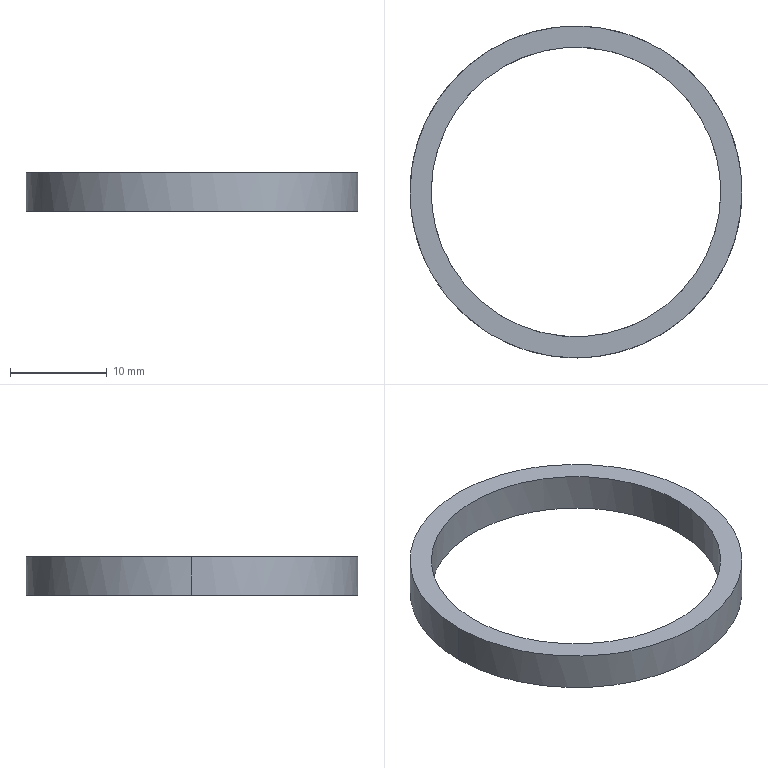Part | STEP file | Resist_ncia-A | 1 solid | 6 faces | box 34.4 x 34.4 x 4 mm | volume 890.436 mm3 | cylinder 4 | plane 2 | commonest cylinder face diameters 30 x2 34.4 x2